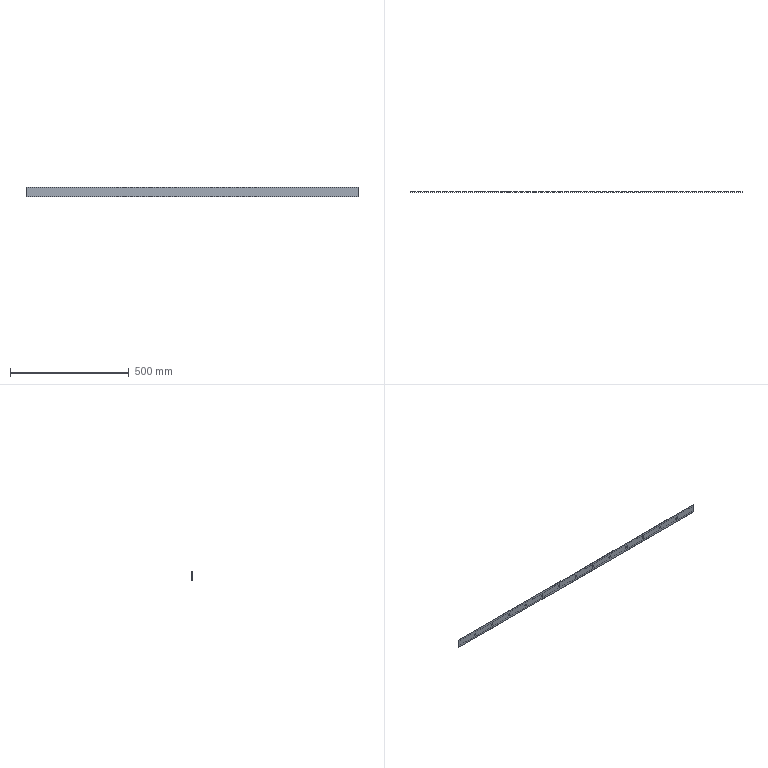Part | SolidWorks | features BaseBody 1 | 1 solid | 1594 faces | box 1400 x 1 x 38 mm | volume 53164 mm3 | plane 1333 | spline 261